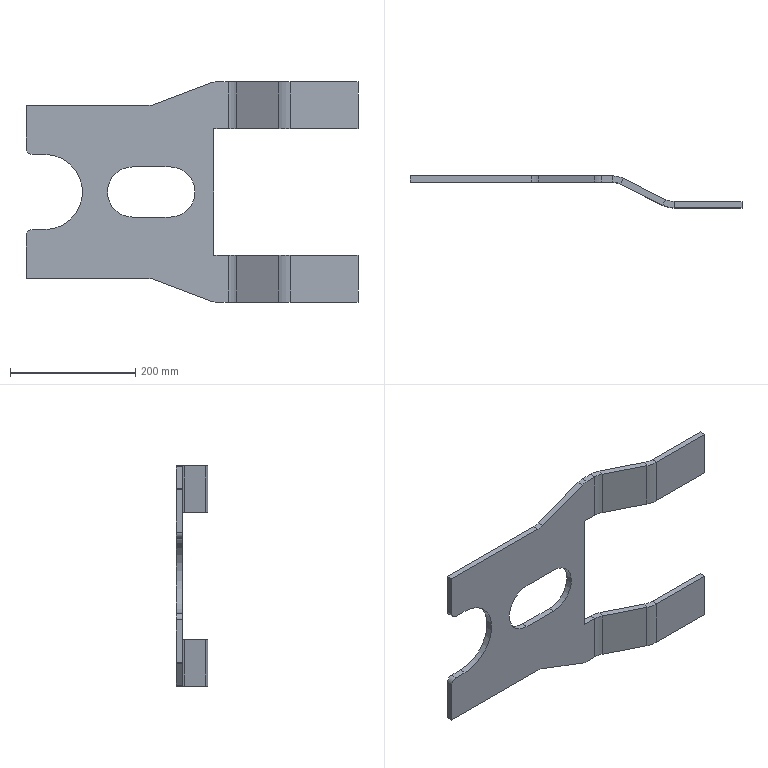Part | SolidWorks | features Fillet 3, Cut 1, Extrusion 1, FlatPattern 1, ICE 1, SheetMetal 1, SolidToSheetMetal 1 | 1 solid | 60 faces | box 530 x 51.056 x 352 mm | volume 1033403 mm3 | plane 43 | cylinder 17 | commonest cylinder face diameters 60 x8 80 x6 20 x2 120 x1